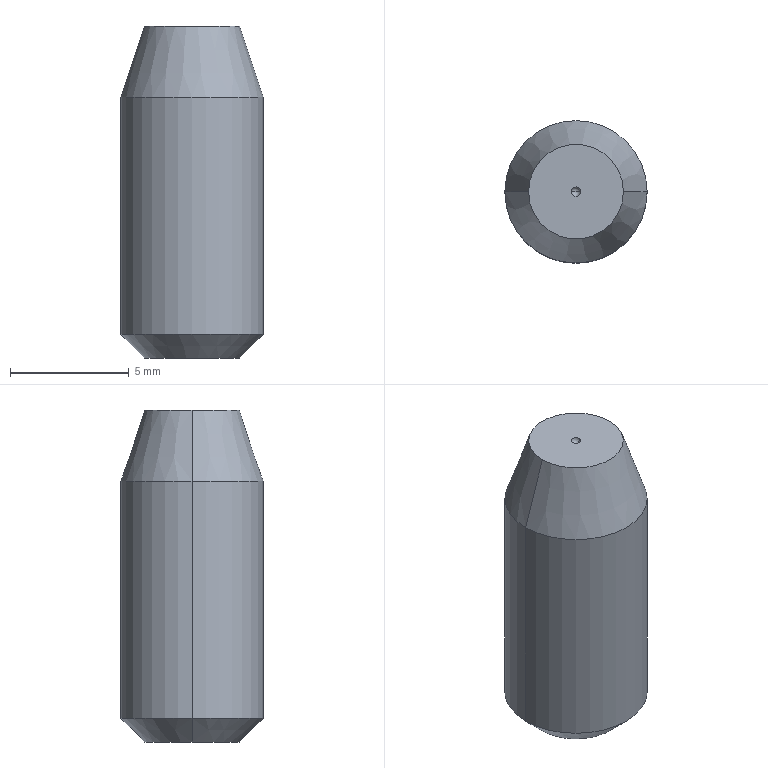Part | STEP file | ASND-0110-Positioning edgeHSG side gTCTF01 | 1 solid | 10 faces | box 6 x 6 x 14 mm | volume 362.314 mm3 | cone 4 | sphere 2 | cylinder 2 | plane 2 | commonest cylinder face diameters 6 x2
STEP:
#1=CARTESIAN_POINT('',(0.,0.,0.));
#2=DIRECTION('',(0.,0.,1.));
#3=DIRECTION('',(1.,0.,0.));
#4=AXIS2_PLACEMENT_3D('',#1,#2,#3);
#5=CARTESIAN_POINT('',(0.2,0.,9.));
#6=VERTEX_POINT('',#5);
#7=CARTESIAN_POINT('',(0.,-0.2,9.));
#8=VERTEX_POINT('',#7);
#9=CARTESIAN_POINT('',(0.,0.,9.));
#10=DIRECTION('',(0.,0.,-1.));
#11=DIRECTION('',(-1.,0.,0.));
#12=AXIS2_PLACEMENT_3D('',#9,#10,#11);
#13=CIRCLE('',#12,0.2);
#14=CARTESIAN_POINT('',(0.,0.,9.));
#15=DIRECTION('',(0.,1.,0.));
#16=DIRECTION('',(1.,0.,0.));
#17=AXIS2_PLACEMENT_3D('',#14,#15,#16);
#18=SPHERICAL_SURFACE('',#17,0.2);
#19=CARTESIAN_POINT('',(0.,3.142));
#20=DIRECTION('',(0.,-1.));
#21=VECTOR('',#20,1.);
#22=LINE('',#19,#21);
#23=(GEOMETRIC_REPRESENTATION_CONTEXT(2)PARAMETRIC_REPRESENTATION_CONTEXT()REPRESENTATION_CONTEXT('',''));
#24=DEFINITIONAL_REPRESENTATION('',(#22),#23);
#25=PCURVE('',#18,#24);
#26=CARTESIAN_POINT('',(0.,0.,9.));
#27=DIRECTION('',(0.,0.,1.));
#28=DIRECTION('',(0.7071,0.7071,0.));
#29=AXIS2_PLACEMENT_3D('',#26,#27,#28);
#30=PLANE('',#29);
#31=CARTESIAN_POINT('',(-0.1414,0.1414));
#32=CARTESIAN_POINT('',(0.1035,0.3864));
#33=CARTESIAN_POINT('',(0.1932,0.05176));
#34=CARTESIAN_POINT('',(0.2828,-0.2828));
#35=CARTESIAN_POINT('',(-0.05176,-0.1932));
#36=CARTESIAN_POINT('',(-0.3864,-0.1035));
#37=CARTESIAN_POINT('',(-0.1414,0.1414));
#38=(BOUNDED_CURVE()B_SPLINE_CURVE(2,(#31,#32,#33,#34,#35,#36,#37),.UNSPECIFIED.,.T.,.F.)B_SPLINE_CURVE_WITH_KNOTS((1,2,2,2,2,1),(-2.094,0.,2.094,4.189,6.283,8.378),.UNSPECIFIED.)CURVE()GEOMETRIC_REPRESENTATION_ITEM()RATIONAL_B_SPLINE_CURVE((1.,0.5,1.,0.5,1.,0.5,1.))REPRESENTATION_ITEM(''));
#39=(GEOMETRIC_REPRESENTATION_CONTEXT(2)PARAMETRIC_REPRESENTATION_CONTEXT()REPRESENTATION_CONTEXT('',''));
#40=DEFINITIONAL_REPRESENTATION('',(#38),#39);
#41=PCURVE('',#30,#40);
#42=SURFACE_CURVE('',#13,(#25,#41),.PCURVE_S1.);
#43=EDGE_CURVE('',#6,#8,#42,.T.);
#44=ORIENTED_EDGE('',*,*,#43,.T.);
#45=CARTESIAN_POINT('',(-0.2,0.,9.));
#46=VERTEX_POINT('',#45);
#47=CARTESIAN_POINT('',(0.,0.,9.));
#48=DIRECTION('',(0.,0.,-1.));
#49=DIRECTION('',(-1.,0.,0.));
#50=AXIS2_PLACEMENT_3D('',#47,#48,#49);
#51=CIRCLE('',#50,0.2);
#52=CARTESIAN_POINT('',(3.142,-1.571));
#53=CARTESIAN_POINT('',(3.142,-1.547));
#54=CARTESIAN_POINT('',(3.142,-1.499));
#55=CARTESIAN_POINT('',(3.142,-1.428));
#56=CARTESIAN_POINT('',(3.142,-1.357));
#57=CARTESIAN_POINT('',(3.142,-1.285));
#58=CARTESIAN_POINT('',(3.142,-1.214));
#59=CARTESIAN_POINT('',(3.142,-1.142));
#60=CARTESIAN_POINT('',(3.142,-1.071));
#61=CARTESIAN_POINT('',(3.142,-0.9996));
#62=CARTESIAN_POINT('',(3.142,-0.9282));
#63=CARTESIAN_POINT('',(3.142,-0.8568));
#64=CARTESIAN_POINT('',(3.142,-0.7854));
#65=CARTESIAN_POINT('',(3.142,-0.714));
#66=CARTESIAN_POINT('',(3.142,-0.6426));
#67=CARTESIAN_POINT('',(3.142,-0.5712));
#68=CARTESIAN_POINT('',(3.142,-0.4998));
#69=CARTESIAN_POINT('',(3.142,-0.4284));
#70=CARTESIAN_POINT('',(3.142,-0.357));
#71=CARTESIAN_POINT('',(3.142,-0.2856));
#72=CARTESIAN_POINT('',(3.142,-0.2142));
#73=CARTESIAN_POINT('',(3.142,-0.1428));
#74=CARTESIAN_POINT('',(3.142,-0.0714));
#75=CARTESIAN_POINT('',(3.142,-0.0238));
#76=CARTESIAN_POINT('',(3.142,0.));
#77=B_SPLINE_CURVE_WITH_KNOTS('',3,(#52,#53,#54,#55,#56,#57,#58,#59,#60,#61,#62,#63,#64,#65,#66,#67,#68,#69,#70,#71,#72,#73,#74,#75,#76),.UNSPECIFIED.,.F.,.F.,(4,1,1,1,1,1,1,1,1,1,1,1,1,1,1,1,1,1,1,1,1,1,4),(4.712,4.784,4.855,4.927,4.998,5.069,5.141,5.212,5.284,5.355,5.426,5.498,5.569,5.641,5.712,5.783,5.855,5.926,5.998,6.069,6.14,6.212,6.283),.QUASI_UNIFORM_KNOTS.);
#78=(GEOMETRIC_REPRESENTATION_CONTEXT(2)PARAMETRIC_REPRESENTATION_CONTEXT()REPRESENTATION_CONTEXT('',''));
#79=DEFINITIONAL_REPRESENTATION('',(#77),#78);
#80=PCURVE('',#18,#79);
#81=CARTESIAN_POINT('',(-0.1414,0.1414));
#82=CARTESIAN_POINT('',(0.1035,0.3864));
#83=CARTESIAN_POINT('',(0.1932,0.05176));
#84=CARTESIAN_POINT('',(0.2828,-0.2828));
#85=CARTESIAN_POINT('',(-0.05176,-0.1932));
#86=CARTESIAN_POINT('',(-0.3864,-0.1035));
#87=CARTESIAN_POINT('',(-0.1414,0.1414));
#88=(BOUNDED_CURVE()B_SPLINE_CURVE(2,(#81,#82,#83,#84,#85,#86,#87),.UNSPECIFIED.,.T.,.F.)B_SPLINE_CURVE_WITH_KNOTS((1,2,2,2,2,1),(-2.094,0.,2.094,4.189,6.283,8.378),.UNSPECIFIED.)CURVE()GEOMETRIC_REPRESENTATION_ITEM()RATIONAL_B_SPLINE_CURVE((1.,0.5,1.,0.5,1.,0.5,1.))REPRESENTATION_ITEM(''));
#89=(GEOMETRIC_REPRESENTATION_CONTEXT(2)PARAMETRIC_REPRESENTATION_CONTEXT()REPRESENTATION_CONTEXT('',''));
#90=DEFINITIONAL_REPRESENTATION('',(#88),#89);
#91=PCURVE('',#30,#90);
#92=SURFACE_CURVE('',#51,(#80,#91),.PCURVE_S1.);
#93=EDGE_CURVE('',#8,#46,#92,.T.);
#94=ORIENTED_EDGE('',*,*,#93,.T.);
#95=CARTESIAN_POINT('',(0.,0.,8.8));
#96=VERTEX_POINT('',#95);
#97=CARTESIAN_POINT('',(0.,0.,9.));
#98=DIRECTION('',(0.,1.,0.));
#99=DIRECTION('',(-1.,0.,0.));
#100=AXIS2_PLACEMENT_3D('',#97,#98,#99);
#101=CIRCLE('',#100,0.2);
#102=CARTESIAN_POINT('',(-3.142,0.));
#103=DIRECTION('',(1.,0.));
#104=VECTOR('',#103,1.);
#105=LINE('',#102,#104);
#106=(GEOMETRIC_REPRESENTATION_CONTEXT(2)PARAMETRIC_REPRESENTATION_CONTEXT()REPRESENTATION_CONTEXT('',''));
#107=DEFINITIONAL_REPRESENTATION('',(#105),#106);
#108=PCURVE('',#18,#107);
#109=CARTESIAN_POINT('',(0.,0.,9.));
#110=DIRECTION('',(0.,1.,0.));
#111=DIRECTION('',(1.,0.,0.));
#112=AXIS2_PLACEMENT_3D('',#109,#110,#111);
#113=SPHERICAL_SURFACE('',#112,0.2);
#114=CARTESIAN_POINT('',(-3.142,0.));
#115=DIRECTION('',(1.,0.));
#116=VECTOR('',#115,1.);
#117=LINE('',#114,#116);
#118=(GEOMETRIC_REPRESENTATION_CONTEXT(2)PARAMETRIC_REPRESENTATION_CONTEXT()REPRESENTATION_CONTEXT('',''));
#119=DEFINITIONAL_REPRESENTATION('',(#117),#118);
#120=PCURVE('',#113,#119);
#121=SURFACE_CURVE('',#101,(#108,#120),.PCURVE_S1.);
#122=EDGE_CURVE('',#96,#46,#121,.T.);
#123=ORIENTED_EDGE('',*,*,#122,.F.);
#124=CARTESIAN_POINT('',(0.,0.,9.));
#125=DIRECTION('',(0.,-1.,0.));
#126=DIRECTION('',(0.,0.,-1.));
#127=AXIS2_PLACEMENT_3D('',#124,#125,#126);
#128=CIRCLE('',#127,0.2);
#129=CARTESIAN_POINT('',(1.571,0.));
#130=DIRECTION('',(-1.,0.));
#131=VECTOR('',#130,1.);
#132=LINE('',#129,#131);
#133=(GEOMETRIC_REPRESENTATION_CONTEXT(2)PARAMETRIC_REPRESENTATION_CONTEXT()REPRESENTATION_CONTEXT('',''));
#134=DEFINITIONAL_REPRESENTATION('',(#132),#133);
#135=PCURVE('',#18,#134);
#136=CARTESIAN_POINT('',(1.571,0.));
#137=DIRECTION('',(-1.,0.));
#138=VECTOR('',#137,1.);
#139=LINE('',#136,#138);
#140=(GEOMETRIC_REPRESENTATION_CONTEXT(2)PARAMETRIC_REPRESENTATION_CONTEXT()REPRESENTATION_CONTEXT('',''));
#141=DEFINITIONAL_REPRESENTATION('',(#139),#140);
#142=PCURVE('',#113,#141);
#143=SURFACE_CURVE('',#128,(#135,#142),.PCURVE_S1.);
#144=EDGE_CURVE('',#96,#6,#143,.T.);
#145=ORIENTED_EDGE('',*,*,#144,.T.);
#146=EDGE_LOOP('',(#44,#94,#123,#145));
#147=FACE_BOUND('',#146,.F.);
#148=ADVANCED_FACE('',(#147),#18,.F.);
#149=CARTESIAN_POINT('',(2.,0.,9.));
#150=VERTEX_POINT('',#149);
#151=CARTESIAN_POINT('',(-2.,0.,9.));
#152=VERTEX_POINT('',#151);
#153=CARTESIAN_POINT('',(0.,0.,9.));
#154=DIRECTION('',(0.,0.,1.));
#155=DIRECTION('',(1.,0.,0.));
#156=AXIS2_PLACEMENT_3D('',#153,#154,#155);
#157=CIRCLE('',#156,2.);
#158=CARTESIAN_POINT('',(0.,0.,9.));
#159=DIRECTION('',(0.,0.,-1.));
#160=DIRECTION('',(-1.,0.,0.));
#161=AXIS2_PLACEMENT_3D('',#158,#159,#160);
#162=CONICAL_SURFACE('',#161,2.,0.3218);
#163=CARTESIAN_POINT('',(3.142,0.));
#164=DIRECTION('',(-1.,0.));
#165=VECTOR('',#164,1.);
#166=LINE('',#163,#165);
#167=(GEOMETRIC_REPRESENTATION_CONTEXT(2)PARAMETRIC_REPRESENTATION_CONTEXT()REPRESENTATION_CONTEXT('',''));
#168=DEFINITIONAL_REPRESENTATION('',(#166),#167);
#169=PCURVE('',#162,#168);
#170=CARTESIAN_POINT('',(0.,0.));
#171=DIRECTION('',(0.7071,-0.7071));
#172=AXIS2_PLACEMENT_2D('',#170,#171);
#173=CIRCLE('',#172,2.);
#174=(GEOMETRIC_REPRESENTATION_CONTEXT(2)PARAMETRIC_REPRESENTATION_CONTEXT()REPRESENTATION_CONTEXT('',''));
#175=DEFINITIONAL_REPRESENTATION('',(#173),#174);
#176=PCURVE('',#30,#175);
#177=SURFACE_CURVE('',#157,(#169,#176),.PCURVE_S1.);
#178=EDGE_CURVE('',#150,#152,#177,.T.);
#179=ORIENTED_EDGE('',*,*,#178,.F.);
#180=CARTESIAN_POINT('',(3.,0.,6.));
#181=VERTEX_POINT('',#180);
#182=CARTESIAN_POINT('',(2.,0.,9.));
#183=DIRECTION('',(0.3162,0.,-0.9487));
#184=VECTOR('',#183,1.);
#185=LINE('',#182,#184);
#186=CARTESIAN_POINT('',(3.142,0.));
#187=DIRECTION('',(0.,1.));
#188=VECTOR('',#187,1.);
#189=LINE('',#186,#188);
#190=(GEOMETRIC_REPRESENTATION_CONTEXT(2)PARAMETRIC_REPRESENTATION_CONTEXT()REPRESENTATION_CONTEXT('',''));
#191=DEFINITIONAL_REPRESENTATION('',(#189),#190);
#192=PCURVE('',#162,#191);
#193=CARTESIAN_POINT('',(0.,0.,9.));
#194=DIRECTION('',(0.,0.,-1.));
#195=DIRECTION('',(-1.,0.,0.));
#196=AXIS2_PLACEMENT_3D('',#193,#194,#195);
#197=CONICAL_SURFACE('',#196,2.,0.3218);
#198=CARTESIAN_POINT('',(3.142,0.));
#199=DIRECTION('',(0.,1.));
#200=VECTOR('',#199,1.);
#201=LINE('',#198,#200);
#202=(GEOMETRIC_REPRESENTATION_CONTEXT(2)PARAMETRIC_REPRESENTATION_CONTEXT()REPRESENTATION_CONTEXT('',''));
#203=DEFINITIONAL_REPRESENTATION('',(#201),#202);
#204=PCURVE('',#197,#203);
#205=SURFACE_CURVE('',#185,(#192,#204),.PCURVE_S1.);
#206=EDGE_CURVE('',#150,#181,#205,.T.);
#207=ORIENTED_EDGE('',*,*,#206,.T.);
#208=CARTESIAN_POINT('',(-3.,0.,6.));
#209=VERTEX_POINT('',#208);
#210=CARTESIAN_POINT('',(0.,0.,6.));
#211=DIRECTION('',(0.,0.,-1.));
#212=DIRECTION('',(1.,0.,0.));
#213=AXIS2_PLACEMENT_3D('',#210,#211,#212);
#214=CIRCLE('',#213,3.);
#215=CARTESIAN_POINT('',(-3.142,3.));
#216=DIRECTION('',(1.,0.));
#217=VECTOR('',#216,1.);
#218=LINE('',#215,#217);
#219=(GEOMETRIC_REPRESENTATION_CONTEXT(2)PARAMETRIC_REPRESENTATION_CONTEXT()REPRESENTATION_CONTEXT('',''));
#220=DEFINITIONAL_REPRESENTATION('',(#218),#219);
#221=PCURVE('',#162,#220);
#222=CARTESIAN_POINT('',(0.,0.,9.));
#223=DIRECTION('',(0.,0.,-1.));
#224=DIRECTION('',(-1.,0.,0.));
#225=AXIS2_PLACEMENT_3D('',#222,#223,#224);
#226=CYLINDRICAL_SURFACE('',#225,3.);
#227=CARTESIAN_POINT('',(-3.142,3.));
#228=DIRECTION('',(1.,0.));
#229=VECTOR('',#228,1.);
#230=LINE('',#227,#229);
#231=(GEOMETRIC_REPRESENTATION_CONTEXT(2)PARAMETRIC_REPRESENTATION_CONTEXT()REPRESENTATION_CONTEXT('',''));
#232=DEFINITIONAL_REPRESENTATION('',(#230),#231);
#233=PCURVE('',#226,#232);
#234=SURFACE_CURVE('',#214,(#221,#233),.PCURVE_S1.);
#235=EDGE_CURVE('',#209,#181,#234,.T.);
#236=ORIENTED_EDGE('',*,*,#235,.F.);
#237=CARTESIAN_POINT('',(-2.,0.,9.));
#238=DIRECTION('',(-0.3162,0.,-0.9487));
#239=VECTOR('',#238,1.);
#240=LINE('',#237,#239);
#241=CARTESIAN_POINT('',(0.,0.));
#242=DIRECTION('',(0.,1.));
#243=VECTOR('',#242,1.);
#244=LINE('',#241,#243);
#245=(GEOMETRIC_REPRESENTATION_CONTEXT(2)PARAMETRIC_REPRESENTATION_CONTEXT()REPRESENTATION_CONTEXT('',''));
#246=DEFINITIONAL_REPRESENTATION('',(#244),#245);
#247=PCURVE('',#162,#246);
#248=CARTESIAN_POINT('',(6.283,0.));
#249=DIRECTION('',(0.,1.));
#250=VECTOR('',#249,1.);
#251=LINE('',#248,#250);
#252=(GEOMETRIC_REPRESENTATION_CONTEXT(2)PARAMETRIC_REPRESENTATION_CONTEXT()REPRESENTATION_CONTEXT('',''));
#253=DEFINITIONAL_REPRESENTATION('',(#251),#252);
#254=PCURVE('',#197,#253);
#255=SURFACE_CURVE('',#240,(#247,#254),.PCURVE_S1.);
#256=EDGE_CURVE('',#152,#209,#255,.T.);
#257=ORIENTED_EDGE('',*,*,#256,.F.);
#258=EDGE_LOOP('',(#179,#207,#236,#257));
#259=FACE_BOUND('',#258,.T.);
#260=ADVANCED_FACE('',(#259),#162,.T.);
#261=CARTESIAN_POINT('',(-2.,0.,-5.));
#262=VERTEX_POINT('',#261);
#263=CARTESIAN_POINT('',(2.,0.,-5.));
#264=VERTEX_POINT('',#263);
#265=CARTESIAN_POINT('',(0.,0.,-5.));
#266=DIRECTION('',(0.,0.,-1.));
#267=DIRECTION('',(-1.,0.,0.));
#268=AXIS2_PLACEMENT_3D('',#265,#266,#267);
#269=CIRCLE('',#268,2.);
#270=CARTESIAN_POINT('',(0.,0.,-5.));
#271=DIRECTION('',(0.,0.,1.));
#272=DIRECTION('',(1.,0.,0.));
#273=AXIS2_PLACEMENT_3D('',#270,#271,#272);
#274=CONICAL_SURFACE('',#273,2.,0.7854);
#275=CARTESIAN_POINT('',(3.142,0.));
#276=DIRECTION('',(-1.,0.));
#277=VECTOR('',#276,1.);
#278=LINE('',#275,#277);
#279=(GEOMETRIC_REPRESENTATION_CONTEXT(2)PARAMETRIC_REPRESENTATION_CONTEXT()REPRESENTATION_CONTEXT('',''));
#280=DEFINITIONAL_REPRESENTATION('',(#278),#279);
#281=PCURVE('',#274,#280);
#282=CARTESIAN_POINT('',(0.,0.,-5.));
#283=DIRECTION('',(0.,0.,-1.));
#284=DIRECTION('',(0.7071,0.7071,0.));
#285=AXIS2_PLACEMENT_3D('',#282,#283,#284);
#286=PLANE('',#285);
#287=CARTESIAN_POINT('',(0.,0.));
#288=DIRECTION('',(-0.7071,-0.7071));
#289=AXIS2_PLACEMENT_2D('',#287,#288);
#290=CIRCLE('',#289,2.);
#291=(GEOMETRIC_REPRESENTATION_CONTEXT(2)PARAMETRIC_REPRESENTATION_CONTEXT()REPRESENTATION_CONTEXT('',''));
#292=DEFINITIONAL_REPRESENTATION('',(#290),#291);
#293=PCURVE('',#286,#292);
#294=SURFACE_CURVE('',#269,(#281,#293),.PCURVE_S1.);
#295=EDGE_CURVE('',#262,#264,#294,.T.);
#296=ORIENTED_EDGE('',*,*,#295,.F.);
#297=CARTESIAN_POINT('',(-3.,0.,-4.));
#298=VERTEX_POINT('',#297);
#299=CARTESIAN_POINT('',(-2.,0.,-5.));
#300=DIRECTION('',(-0.7071,0.,0.7071));
#301=VECTOR('',#300,1.);
#302=LINE('',#299,#301);
#303=CARTESIAN_POINT('',(3.142,0.));
#304=DIRECTION('',(0.,1.));
#305=VECTOR('',#304,1.);
#306=LINE('',#303,#305);
#307=(GEOMETRIC_REPRESENTATION_CONTEXT(2)PARAMETRIC_REPRESENTATION_CONTEXT()REPRESENTATION_CONTEXT('',''));
#308=DEFINITIONAL_REPRESENTATION('',(#306),#307);
#309=PCURVE('',#274,#308);
#310=CARTESIAN_POINT('',(0.,0.,-5.));
#311=DIRECTION('',(0.,0.,1.));
#312=DIRECTION('',(1.,0.,0.));
#313=AXIS2_PLACEMENT_3D('',#310,#311,#312);
#314=CONICAL_SURFACE('',#313,2.,0.7854);
#315=CARTESIAN_POINT('',(3.142,0.));
#316=DIRECTION('',(0.,1.));
#317=VECTOR('',#316,1.);
#318=LINE('',#315,#317);
#319=(GEOMETRIC_REPRESENTATION_CONTEXT(2)PARAMETRIC_REPRESENTATION_CONTEXT()REPRESENTATION_CONTEXT('',''));
#320=DEFINITIONAL_REPRESENTATION('',(#318),#319);
#321=PCURVE('',#314,#320);
#322=SURFACE_CURVE('',#302,(#309,#321),.PCURVE_S1.);
#323=EDGE_CURVE('',#262,#298,#322,.T.);
#324=ORIENTED_EDGE('',*,*,#323,.T.);
#325=CARTESIAN_POINT('',(3.,0.,-4.));
#326=VERTEX_POINT('',#325);
#327=CARTESIAN_POINT('',(0.,0.,-4.));
#328=DIRECTION('',(0.,0.,1.));
#329=DIRECTION('',(-1.,0.,0.));
#330=AXIS2_PLACEMENT_3D('',#327,#328,#329);
#331=CIRCLE('',#330,3.);
#332=CARTESIAN_POINT('',(-3.142,1.));
#333=DIRECTION('',(1.,0.));
#334=VECTOR('',#333,1.);
#335=LINE('',#332,#334);
#336=(GEOMETRIC_REPRESENTATION_CONTEXT(2)PARAMETRIC_REPRESENTATION_CONTEXT()REPRESENTATION_CONTEXT('',''));
#337=DEFINITIONAL_REPRESENTATION('',(#335),#336);
#338=PCURVE('',#274,#337);
#339=CARTESIAN_POINT('',(6.283,13.));
#340=DIRECTION('',(-1.,0.));
#341=VECTOR('',#340,1.);
#342=LINE('',#339,#341);
#343=(GEOMETRIC_REPRESENTATION_CONTEXT(2)PARAMETRIC_REPRESENTATION_CONTEXT()REPRESENTATION_CONTEXT('',''));
#344=DEFINITIONAL_REPRESENTATION('',(#342),#343);
#345=PCURVE('',#226,#344);
#346=SURFACE_CURVE('',#331,(#338,#345),.PCURVE_S1.);
#347=EDGE_CURVE('',#326,#298,#346,.T.);
#348=ORIENTED_EDGE('',*,*,#347,.F.);
#349=CARTESIAN_POINT('',(2.,0.,-5.));
#350=DIRECTION('',(0.7071,0.,0.7071));
#351=VECTOR('',#350,1.);
#352=LINE('',#349,#351);
#353=CARTESIAN_POINT('',(0.,0.));
#354=DIRECTION('',(0.,1.));
#355=VECTOR('',#354,1.);
#356=LINE('',#353,#355);
#357=(GEOMETRIC_REPRESENTATION_CONTEXT(2)PARAMETRIC_REPRESENTATION_CONTEXT()REPRESENTATION_CONTEXT('',''));
#358=DEFINITIONAL_REPRESENTATION('',(#356),#357);
#359=PCURVE('',#274,#358);
#360=CARTESIAN_POINT('',(6.283,0.));
#361=DIRECTION('',(0.,1.));
#362=VECTOR('',#361,1.);
#363=LINE('',#360,#362);
#364=(GEOMETRIC_REPRESENTATION_CONTEXT(2)PARAMETRIC_REPRESENTATION_CONTEXT()REPRESENTATION_CONTEXT('',''));
#365=DEFINITIONAL_REPRESENTATION('',(#363),#364);
#366=PCURVE('',#314,#365);
#367=SURFACE_CURVE('',#352,(#359,#366),.PCURVE_S1.);
#368=EDGE_CURVE('',#264,#326,#367,.T.);
#369=ORIENTED_EDGE('',*,*,#368,.F.);
#370=EDGE_LOOP('',(#296,#324,#348,#369));
#371=FACE_BOUND('',#370,.T.);
#372=ADVANCED_FACE('',(#371),#274,.T.);
#373=ORIENTED_EDGE('',*,*,#235,.T.);
#374=CARTESIAN_POINT('',(3.,0.,9.));
#375=DIRECTION('',(0.,0.,-1.));
#376=VECTOR('',#375,1.);
#377=LINE('',#374,#376);
#378=CARTESIAN_POINT('',(3.142,0.));
#379=DIRECTION('',(0.,1.));
#380=VECTOR('',#379,1.);
#381=LINE('',#378,#380);
#382=(GEOMETRIC_REPRESENTATION_CONTEXT(2)PARAMETRIC_REPRESENTATION_CONTEXT()REPRESENTATION_CONTEXT('',''));
#383=DEFINITIONAL_REPRESENTATION('',(#381),#382);
#384=PCURVE('',#226,#383);
#385=CARTESIAN_POINT('',(0.,0.,9.));
#386=DIRECTION('',(0.,0.,-1.));
#387=DIRECTION('',(-1.,0.,0.));
#388=AXIS2_PLACEMENT_3D('',#385,#386,#387);
#389=CYLINDRICAL_SURFACE('',#388,3.);
#390=CARTESIAN_POINT('',(3.142,0.));
#391=DIRECTION('',(0.,1.));
#392=VECTOR('',#391,1.);
#393=LINE('',#390,#392);
#394=(GEOMETRIC_REPRESENTATION_CONTEXT(2)PARAMETRIC_REPRESENTATION_CONTEXT()REPRESENTATION_CONTEXT('',''));
#395=DEFINITIONAL_REPRESENTATION('',(#393),#394);
#396=PCURVE('',#389,#395);
#397=SURFACE_CURVE('',#377,(#384,#396),.PCURVE_S1.);
#398=EDGE_CURVE('',#181,#326,#397,.T.);
#399=ORIENTED_EDGE('',*,*,#398,.T.);
#400=ORIENTED_EDGE('',*,*,#347,.T.);
#401=CARTESIAN_POINT('',(-3.,0.,9.));
#402=DIRECTION('',(0.,0.,-1.));
#403=VECTOR('',#402,1.);
#404=LINE('',#401,#403);
#405=CARTESIAN_POINT('',(0.,0.));
#406=DIRECTION('',(0.,1.));
#407=VECTOR('',#406,1.);
#408=LINE('',#405,#407);
#409=(GEOMETRIC_REPRESENTATION_CONTEXT(2)PARAMETRIC_REPRESENTATION_CONTEXT()REPRESENTATION_CONTEXT('',''));
#410=DEFINITIONAL_REPRESENTATION('',(#408),#409);
#411=PCURVE('',#226,#410);
#412=CARTESIAN_POINT('',(6.283,0.));
#413=DIRECTION('',(0.,1.));
#414=VECTOR('',#413,1.);
#415=LINE('',#412,#414);
#416=(GEOMETRIC_REPRESENTATION_CONTEXT(2)PARAMETRIC_REPRESENTATION_CONTEXT()REPRESENTATION_CONTEXT('',''));
#417=DEFINITIONAL_REPRESENTATION('',(#415),#416);
#418=PCURVE('',#389,#417);
#419=SURFACE_CURVE('',#404,(#411,#418),.PCURVE_S1.);
#420=EDGE_CURVE('',#209,#298,#419,.T.);
#421=ORIENTED_EDGE('',*,*,#420,.F.);
#422=EDGE_LOOP('',(#373,#399,#400,#421));
#423=FACE_BOUND('',#422,.T.);
#424=ADVANCED_FACE('',(#423),#226,.T.);
#425=CARTESIAN_POINT('',(0.,0.,9.));
#426=DIRECTION('',(0.,0.,1.));
#427=DIRECTION('',(1.,0.,0.));
#428=AXIS2_PLACEMENT_3D('',#425,#426,#427);
#429=CIRCLE('',#428,2.);
#430=CARTESIAN_POINT('',(0.,0.));
#431=DIRECTION('',(0.7071,-0.7071));
#432=AXIS2_PLACEMENT_2D('',#430,#431);
#433=CIRCLE('',#432,2.);
#434=(GEOMETRIC_REPRESENTATION_CONTEXT(2)PARAMETRIC_REPRESENTATION_CONTEXT()REPRESENTATION_CONTEXT('',''));
#435=DEFINITIONAL_REPRESENTATION('',(#433),#434);
#436=PCURVE('',#30,#435);
#437=CARTESIAN_POINT('',(9.425,0.));
#438=DIRECTION('',(-1.,0.));
#439=VECTOR('',#438,1.);
#440=LINE('',#437,#439);
#441=(GEOMETRIC_REPRESENTATION_CONTEXT(2)PARAMETRIC_REPRESENTATION_CONTEXT()REPRESENTATION_CONTEXT('',''));
#442=DEFINITIONAL_REPRESENTATION('',(#440),#441);
#443=PCURVE('',#197,#442);
#444=SURFACE_CURVE('',#429,(#436,#443),.PCURVE_S1.);
#445=EDGE_CURVE('',#152,#150,#444,.T.);
#446=ORIENTED_EDGE('',*,*,#445,.T.);
#447=ORIENTED_EDGE('',*,*,#178,.T.);
#448=EDGE_LOOP('',(#446,#447));
#449=FACE_BOUND('',#448,.T.);
#450=ORIENTED_EDGE('',*,*,#43,.T.);
#451=ORIENTED_EDGE('',*,*,#93,.T.);
#452=CARTESIAN_POINT('',(0.,0.2,9.));
#453=VERTEX_POINT('',#452);
#454=CARTESIAN_POINT('',(0.,0.,9.));
#455=DIRECTION('',(0.,0.,-1.));
#456=DIRECTION('',(-1.,0.,0.));
#457=AXIS2_PLACEMENT_3D('',#454,#455,#456);
#458=CIRCLE('',#457,0.2);
#459=CARTESIAN_POINT('',(-0.1414,0.1414));
#460=CARTESIAN_POINT('',(0.1035,0.3864));
#461=CARTESIAN_POINT('',(0.1932,0.05176));
#462=CARTESIAN_POINT('',(0.2828,-0.2828));
#463=CARTESIAN_POINT('',(-0.05176,-0.1932));
#464=CARTESIAN_POINT('',(-0.3864,-0.1035));
#465=CARTESIAN_POINT('',(-0.1414,0.1414));
#466=(BOUNDED_CURVE()B_SPLINE_CURVE(2,(#459,#460,#461,#462,#463,#464,#465),.UNSPECIFIED.,.T.,.F.)B_SPLINE_CURVE_WITH_KNOTS((1,2,2,2,2,1),(-2.094,0.,2.094,4.189,6.283,8.378),.UNSPECIFIED.)CURVE()GEOMETRIC_REPRESENTATION_ITEM()RATIONAL_B_SPLINE_CURVE((1.,0.5,1.,0.5,1.,0.5,1.))REPRESENTATION_ITEM(''));
#467=(GEOMETRIC_REPRESENTATION_CONTEXT(2)PARAMETRIC_REPRESENTATION_CONTEXT()REPRESENTATION_CONTEXT('',''));
#468=DEFINITIONAL_REPRESENTATION('',(#466),#467);
#469=PCURVE('',#30,#468);
#470=CARTESIAN_POINT('',(3.142,0.));
#471=DIRECTION('',(0.,1.));
#472=VECTOR('',#471,1.);
#473=LINE('',#470,#472);
#474=(GEOMETRIC_REPRESENTATION_CONTEXT(2)PARAMETRIC_REPRESENTATION_CONTEXT()REPRESENTATION_CONTEXT('',''));
#475=DEFINITIONAL_REPRESENTATION('',(#473),#474);
#476=PCURVE('',#113,#475);
#477=SURFACE_CURVE('',#458,(#469,#476),.PCURVE_S1.);
#478=EDGE_CURVE('',#46,#453,#477,.T.);
#479=ORIENTED_EDGE('',*,*,#478,.T.);
#480=CARTESIAN_POINT('',(0.,0.,9.));
#481=DIRECTION('',(0.,0.,-1.));
#482=DIRECTION('',(-1.,0.,0.));
#483=AXIS2_PLACEMENT_3D('',#480,#481,#482);
#484=CIRCLE('',#483,0.2);
#485=CARTESIAN_POINT('',(-0.1414,0.1414));
#486=CARTESIAN_POINT('',(0.1035,0.3864));
#487=CARTESIAN_POINT('',(0.1932,0.05176));
#488=CARTESIAN_POINT('',(0.2828,-0.2828));
#489=CARTESIAN_POINT('',(-0.05176,-0.1932));
#490=CARTESIAN_POINT('',(-0.3864,-0.1035));
#491=CARTESIAN_POINT('',(-0.1414,0.1414));
#492=(BOUNDED_CURVE()B_SPLINE_CURVE(2,(#485,#486,#487,#488,#489,#490,#491),.UNSPECIFIED.,.T.,.F.)B_SPLINE_CURVE_WITH_KNOTS((1,2,2,2,2,1),(-2.094,0.,2.094,4.189,6.283,8.378),.UNSPECIFIED.)CURVE()GEOMETRIC_REPRESENTATION_ITEM()RATIONAL_B_SPLINE_CURVE((1.,0.5,1.,0.5,1.,0.5,1.))REPRESENTATION_ITEM(''));
#493=(GEOMETRIC_REPRESENTATION_CONTEXT(2)PARAMETRIC_REPRESENTATION_CONTEXT()REPRESENTATION_CONTEXT('',''));
#494=DEFINITIONAL_REPRESENTATION('',(#492),#493);
#495=PCURVE('',#30,#494);
#496=CARTESIAN_POINT('',(0.,1.571));
#497=CARTESIAN_POINT('',(0.,1.547));
#498=CARTESIAN_POINT('',(0.,1.499));
#499=CARTESIAN_POINT('',(0.,1.428));
#500=CARTESIAN_POINT('',(0.,1.357));
#501=CARTESIAN_POINT('',(0.,1.285));
#502=CARTESIAN_POINT('',(0.,1.214));
#503=CARTESIAN_POINT('',(0.,1.142));
#504=CARTESIAN_POINT('',(0.,1.071));
#505=CARTESIAN_POINT('',(0.,0.9996));
#506=CARTESIAN_POINT('',(0.,0.9282));
#507=CARTESIAN_POINT('',(0.,0.8568));
#508=CARTESIAN_POINT('',(0.,0.7854));
#509=CARTESIAN_POINT('',(0.,0.714));
#510=CARTESIAN_POINT('',(0.,0.6426));
#511=CARTESIAN_POINT('',(0.,0.5712));
#512=CARTESIAN_POINT('',(0.,0.4998));
#513=CARTESIAN_POINT('',(0.,0.4284));
#514=CARTESIAN_POINT('',(0.,0.357));
#515=CARTESIAN_POINT('',(0.,0.2856));
#516=CARTESIAN_POINT('',(0.,0.2142));
#517=CARTESIAN_POINT('',(0.,0.1428));
#518=CARTESIAN_POINT('',(0.,0.0714));
#519=CARTESIAN_POINT('',(0.,0.0238));
#520=CARTESIAN_POINT('',(0.,0.));
#521=B_SPLINE_CURVE_WITH_KNOTS('',3,(#496,#497,#498,#499,#500,#501,#502,#503,#504,#505,#506,#507,#508,#509,#510,#511,#512,#513,#514,#515,#516,#517,#518,#519,#520),.UNSPECIFIED.,.F.,.F.,(4,1,1,1,1,1,1,1,1,1,1,1,1,1,1,1,1,1,1,1,1,1,4),(1.571,1.642,1.714,1.785,1.856,1.928,1.999,2.071,2.142,2.213,2.285,2.356,2.428,2.499,2.57,2.642,2.713,2.785,2.856,2.927,2.999,3.07,3.142),.QUASI_UNIFORM_KNOTS.);
#522=(GEOMETRIC_REPRESENTATION_CONTEXT(2)PARAMETRIC_REPRESENTATION_CONTEXT()REPRESENTATION_CONTEXT('',''));
#523=DEFINITIONAL_REPRESENTATION('',(#521),#522);
#524=PCURVE('',#113,#523);
#525=SURFACE_CURVE('',#484,(#495,#524),.PCURVE_S1.);
#526=EDGE_CURVE('',#453,#6,#525,.T.);
#527=ORIENTED_EDGE('',*,*,#526,.T.);
#528=EDGE_LOOP('',(#450,#451,#479,#527));
#529=FACE_BOUND('',#528,.T.);
#530=ADVANCED_FACE('',(#449,#529),#30,.T.);
#531=ORIENTED_EDGE('',*,*,#398,.F.);
#532=CARTESIAN_POINT('',(0.,0.,6.));
#533=DIRECTION('',(0.,0.,-1.));
#534=DIRECTION('',(1.,0.,0.));
#535=AXIS2_PLACEMENT_3D('',#532,#533,#534);
#536=CIRCLE('',#535,3.);
#537=CARTESIAN_POINT('',(3.142,3.));
#538=DIRECTION('',(1.,0.));
#539=VECTOR('',#538,1.);
#540=LINE('',#537,#539);
#541=(GEOMETRIC_REPRESENTATION_CONTEXT(2)PARAMETRIC_REPRESENTATION_CONTEXT()REPRESENTATION_CONTEXT('',''));
#542=DEFINITIONAL_REPRESENTATION('',(#540),#541);
#543=PCURVE('',#389,#542);
#544=CARTESIAN_POINT('',(3.142,3.));
#545=DIRECTION('',(1.,0.));
#546=VECTOR('',#545,1.);
#547=LINE('',#544,#546);
#548=(GEOMETRIC_REPRESENTATION_CONTEXT(2)PARAMETRIC_REPRESENTATION_CONTEXT()REPRESENTATION_CONTEXT('',''));
#549=DEFINITIONAL_REPRESENTATION('',(#547),#548);
#550=PCURVE('',#197,#549);
#551=SURFACE_CURVE('',#536,(#543,#550),.PCURVE_S1.);
#552=EDGE_CURVE('',#181,#209,#551,.T.);
#553=ORIENTED_EDGE('',*,*,#552,.T.);
#554=ORIENTED_EDGE('',*,*,#420,.T.);
#555=CARTESIAN_POINT('',(0.,0.,-4.));
#556=DIRECTION('',(0.,0.,1.));
#557=DIRECTION('',(-1.,0.,0.));
#558=AXIS2_PLACEMENT_3D('',#555,#556,#557);
#559=CIRCLE('',#558,3.);
#560=CARTESIAN_POINT('',(6.283,13.));
#561=DIRECTION('',(-1.,0.));
#562=VECTOR('',#561,1.);
#563=LINE('',#560,#562);
#564=(GEOMETRIC_REPRESENTATION_CONTEXT(2)PARAMETRIC_REPRESENTATION_CONTEXT()REPRESENTATION_CONTEXT('',''));
#565=DEFINITIONAL_REPRESENTATION('',(#563),#564);
#566=PCURVE('',#389,#565);
#567=CARTESIAN_POINT('',(3.142,1.));
#568=DIRECTION('',(1.,0.));
#569=VECTOR('',#568,1.);
#570=LINE('',#567,#569);
#571=(GEOMETRIC_REPRESENTATION_CONTEXT(2)PARAMETRIC_REPRESENTATION_CONTEXT()REPRESENTATION_CONTEXT('',''));
#572=DEFINITIONAL_REPRESENTATION('',(#570),#571);
#573=PCURVE('',#314,#572);
#574=SURFACE_CURVE('',#559,(#566,#573),.PCURVE_S1.);
#575=EDGE_CURVE('',#298,#326,#574,.T.);
#576=ORIENTED_EDGE('',*,*,#575,.T.);
#577=EDGE_LOOP('',(#531,#553,#554,#576));
#578=FACE_BOUND('',#577,.T.);
#579=ADVANCED_FACE('',(#578),#389,.T.);
#580=CARTESIAN_POINT('',(0.,0.,-5.));
#581=DIRECTION('',(0.,0.,-1.));
#582=DIRECTION('',(-1.,0.,0.));
#583=AXIS2_PLACEMENT_3D('',#580,#581,#582);
#584=CIRCLE('',#583,2.);
#585=CARTESIAN_POINT('',(0.,0.));
#586=DIRECTION('',(-0.7071,-0.7071));
#587=AXIS2_PLACEMENT_2D('',#585,#586);
#588=CIRCLE('',#587,2.);
#589=(GEOMETRIC_REPRESENTATION_CONTEXT(2)PARAMETRIC_REPRESENTATION_CONTEXT()REPRESENTATION_CONTEXT('',''));
#590=DEFINITIONAL_REPRESENTATION('',(#588),#589);
#591=PCURVE('',#286,#590);
#592=CARTESIAN_POINT('',(9.425,0.));
#593=DIRECTION('',(-1.,0.));
#594=VECTOR('',#593,1.);
#595=LINE('',#592,#594);
#596=(GEOMETRIC_REPRESENTATION_CONTEXT(2)PARAMETRIC_REPRESENTATION_CONTEXT()REPRESENTATION_CONTEXT('',''));
#597=DEFINITIONAL_REPRESENTATION('',(#595),#596);
#598=PCURVE('',#314,#597);
#599=SURFACE_CURVE('',#584,(#591,#598),.PCURVE_S1.);
#600=EDGE_CURVE('',#264,#262,#599,.T.);
#601=ORIENTED_EDGE('',*,*,#600,.T.);
#602=ORIENTED_EDGE('',*,*,#295,.T.);
#603=EDGE_LOOP('',(#601,#602));
#604=FACE_BOUND('',#603,.T.);
#605=ADVANCED_FACE('',(#604),#286,.T.);
#606=ORIENTED_EDGE('',*,*,#323,.F.);
#607=ORIENTED_EDGE('',*,*,#600,.F.);
#608=ORIENTED_EDGE('',*,*,#368,.T.);
#609=ORIENTED_EDGE('',*,*,#575,.F.);
#610=EDGE_LOOP('',(#606,#607,#608,#609));
#611=FACE_BOUND('',#610,.T.);
#612=ADVANCED_FACE('',(#611),#314,.T.);
#613=ORIENTED_EDGE('',*,*,#206,.F.);
#614=ORIENTED_EDGE('',*,*,#445,.F.);
#615=ORIENTED_EDGE('',*,*,#256,.T.);
#616=ORIENTED_EDGE('',*,*,#552,.F.);
#617=EDGE_LOOP('',(#613,#614,#615,#616));
#618=FACE_BOUND('',#617,.T.);
#619=ADVANCED_FACE('',(#618),#197,.T.);
#620=ORIENTED_EDGE('',*,*,#478,.T.);
#621=ORIENTED_EDGE('',*,*,#526,.T.);
#622=ORIENTED_EDGE('',*,*,#144,.F.);
#623=ORIENTED_EDGE('',*,*,#122,.T.);
#624=EDGE_LOOP('',(#620,#621,#622,#623));
#625=FACE_BOUND('',#624,.F.);
#626=ADVANCED_FACE('',(#625),#113,.F.);
#627=CLOSED_SHELL('',(#148,#260,#372,#424,#530,#579,#605,#612,#619,#626));
#628=MANIFOLD_SOLID_BREP('',#627);
#629=(LENGTH_UNIT()NAMED_UNIT(*)SI_UNIT(.MILLI.,.METRE.));
#630=UNCERTAINTY_MEASURE_WITH_UNIT(LENGTH_MEASURE(0.0000001),#629,'','');
#631=(NAMED_UNIT(*)PLANE_ANGLE_UNIT()SI_UNIT($,.RADIAN.));
#632=(NAMED_UNIT(*)SI_UNIT($,.STERADIAN.)SOLID_ANGLE_UNIT());
#633=(GEOMETRIC_REPRESENTATION_CONTEXT(3)GLOBAL_UNCERTAINTY_ASSIGNED_CONTEXT((#630))GLOBAL_UNIT_ASSIGNED_CONTEXT((#629,#631,#632))REPRESENTATION_CONTEXT('',''));
#634=ADVANCED_BREP_SHAPE_REPRESENTATION('',(#4,#628),#633);